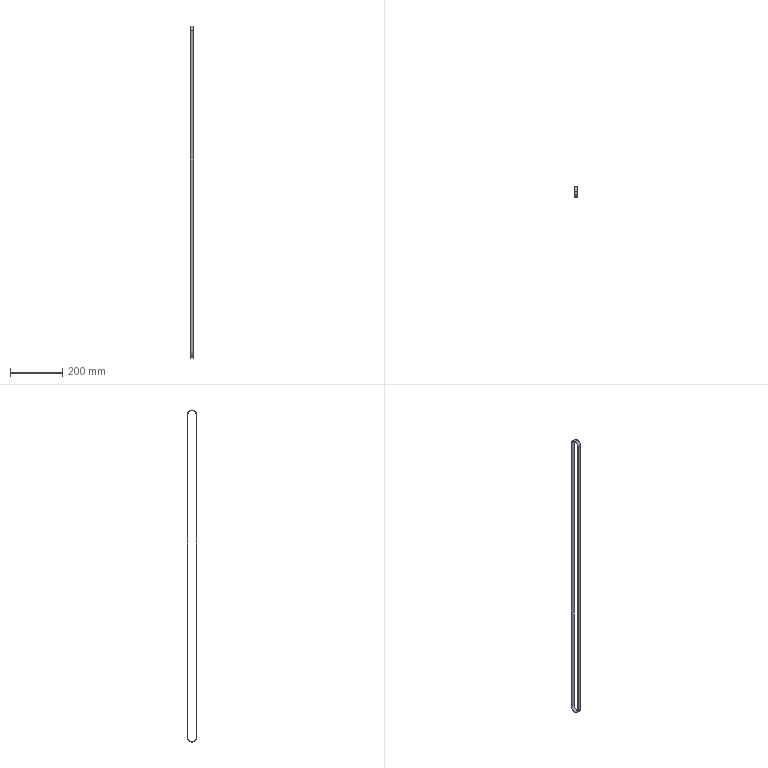Part | STEP file | 0243_101_Belt_050-L-0396A-J | 1 solid | 12 faces | box 13.5 x 37.6 x 1267 mm | volume 69386 mm3 | cylinder 6 | plane 6 | commonest cylinder face diameters 33.6 x3 37.6 x3
STEP:
#1=CARTESIAN_POINT('',(0.,0.,0.));
#2=DIRECTION('',(0.,0.,1.));
#3=DIRECTION('',(1.,0.,0.));
#4=AXIS2_PLACEMENT_3D('',#1,#2,#3);
#5=CARTESIAN_POINT('',(6.75,16.8,0.));
#6=VERTEX_POINT('',#5);
#7=CARTESIAN_POINT('',(-6.75,16.8,0.));
#8=VERTEX_POINT('',#7);
#9=CARTESIAN_POINT('',(6.75,16.8,0.));
#10=DIRECTION('',(-1.,0.,0.));
#11=VECTOR('',#10,1.);
#12=LINE('',#9,#11);
#13=CARTESIAN_POINT('',(6.75,0.,0.));
#14=DIRECTION('',(-1.,0.,0.));
#15=DIRECTION('',(0.,0.,1.));
#16=AXIS2_PLACEMENT_3D('',#13,#14,#15);
#17=CYLINDRICAL_SURFACE('',#16,16.8);
#18=CARTESIAN_POINT('',(1.571,0.));
#19=DIRECTION('',(0.,1.));
#20=VECTOR('',#19,1.);
#21=LINE('',#18,#20);
#22=(GEOMETRIC_REPRESENTATION_CONTEXT(2)PARAMETRIC_REPRESENTATION_CONTEXT()REPRESENTATION_CONTEXT('',''));
#23=DEFINITIONAL_REPRESENTATION('',(#21),#22);
#24=PCURVE('',#17,#23);
#25=CARTESIAN_POINT('',(6.75,16.8,0.));
#26=DIRECTION('',(0.,-1.,0.));
#27=DIRECTION('',(0.,0.,-1.));
#28=AXIS2_PLACEMENT_3D('',#25,#26,#27);
#29=PLANE('',#28);
#30=CARTESIAN_POINT('',(0.,0.));
#31=DIRECTION('',(0.,-1.));
#32=VECTOR('',#31,1.);
#33=LINE('',#30,#32);
#34=(GEOMETRIC_REPRESENTATION_CONTEXT(2)PARAMETRIC_REPRESENTATION_CONTEXT()REPRESENTATION_CONTEXT('',''));
#35=DEFINITIONAL_REPRESENTATION('',(#33),#34);
#36=PCURVE('',#29,#35);
#37=SURFACE_CURVE('',#12,(#24,#36),.PCURVE_S1.);
#38=EDGE_CURVE('',#6,#8,#37,.T.);
#39=ORIENTED_EDGE('',*,*,#38,.T.);
#40=CARTESIAN_POINT('',(-6.75,0.,16.8));
#41=VERTEX_POINT('',#40);
#42=CARTESIAN_POINT('',(-6.75,0.,0.));
#43=DIRECTION('',(1.,0.,0.));
#44=DIRECTION('',(0.,0.,-1.));
#45=AXIS2_PLACEMENT_3D('',#42,#43,#44);
#46=CIRCLE('',#45,16.8);
#47=CARTESIAN_POINT('',(3.142,13.5));
#48=DIRECTION('',(-1.,0.));
#49=VECTOR('',#48,1.);
#50=LINE('',#47,#49);
#51=(GEOMETRIC_REPRESENTATION_CONTEXT(2)PARAMETRIC_REPRESENTATION_CONTEXT()REPRESENTATION_CONTEXT('',''));
#52=DEFINITIONAL_REPRESENTATION('',(#50),#51);
#53=PCURVE('',#17,#52);
#54=CARTESIAN_POINT('',(-6.75,0.,0.));
#55=DIRECTION('',(1.,0.,0.));
#56=DIRECTION('',(0.,0.,-1.));
#57=AXIS2_PLACEMENT_3D('',#54,#55,#56);
#58=PLANE('',#57);
#59=CARTESIAN_POINT('',(0.,0.));
#60=DIRECTION('',(1.,0.));
#61=AXIS2_PLACEMENT_2D('',#59,#60);
#62=CIRCLE('',#61,16.8);
#63=(GEOMETRIC_REPRESENTATION_CONTEXT(2)PARAMETRIC_REPRESENTATION_CONTEXT()REPRESENTATION_CONTEXT('',''));
#64=DEFINITIONAL_REPRESENTATION('',(#62),#63);
#65=PCURVE('',#58,#64);
#66=SURFACE_CURVE('',#46,(#53,#65),.PCURVE_S1.);
#67=EDGE_CURVE('',#8,#41,#66,.T.);
#68=ORIENTED_EDGE('',*,*,#67,.T.);
#69=CARTESIAN_POINT('',(6.75,0.,16.8));
#70=VERTEX_POINT('',#69);
#71=CARTESIAN_POINT('',(6.75,0.,16.8));
#72=DIRECTION('',(-1.,0.,0.));
#73=VECTOR('',#72,1.);
#74=LINE('',#71,#73);
#75=CARTESIAN_POINT('',(0.,0.));
#76=DIRECTION('',(0.,1.));
#77=VECTOR('',#76,1.);
#78=LINE('',#75,#77);
#79=(GEOMETRIC_REPRESENTATION_CONTEXT(2)PARAMETRIC_REPRESENTATION_CONTEXT()REPRESENTATION_CONTEXT('',''));
#80=DEFINITIONAL_REPRESENTATION('',(#78),#79);
#81=PCURVE('',#17,#80);
#82=CARTESIAN_POINT('',(6.75,0.,0.));
#83=DIRECTION('',(-1.,0.,0.));
#84=DIRECTION('',(0.,0.,1.));
#85=AXIS2_PLACEMENT_3D('',#82,#83,#84);
#86=CYLINDRICAL_SURFACE('',#85,16.8);
#87=CARTESIAN_POINT('',(6.283,0.));
#88=DIRECTION('',(0.,1.));
#89=VECTOR('',#88,1.);
#90=LINE('',#87,#89);
#91=(GEOMETRIC_REPRESENTATION_CONTEXT(2)PARAMETRIC_REPRESENTATION_CONTEXT()REPRESENTATION_CONTEXT('',''));
#92=DEFINITIONAL_REPRESENTATION('',(#90),#91);
#93=PCURVE('',#86,#92);
#94=SURFACE_CURVE('',#74,(#81,#93),.PCURVE_S1.);
#95=EDGE_CURVE('',#70,#41,#94,.T.);
#96=ORIENTED_EDGE('',*,*,#95,.F.);
#97=CARTESIAN_POINT('',(6.75,0.,0.));
#98=DIRECTION('',(1.,0.,0.));
#99=DIRECTION('',(0.,0.,-1.));
#100=AXIS2_PLACEMENT_3D('',#97,#98,#99);
#101=CIRCLE('',#100,16.8);
#102=CARTESIAN_POINT('',(3.142,0.));
#103=DIRECTION('',(-1.,0.));
#104=VECTOR('',#103,1.);
#105=LINE('',#102,#104);
#106=(GEOMETRIC_REPRESENTATION_CONTEXT(2)PARAMETRIC_REPRESENTATION_CONTEXT()REPRESENTATION_CONTEXT('',''));
#107=DEFINITIONAL_REPRESENTATION('',(#105),#106);
#108=PCURVE('',#17,#107);
#109=CARTESIAN_POINT('',(6.75,0.,0.));
#110=DIRECTION('',(1.,0.,0.));
#111=DIRECTION('',(0.,0.,-1.));
#112=AXIS2_PLACEMENT_3D('',#109,#110,#111);
#113=PLANE('',#112);
#114=CARTESIAN_POINT('',(0.,0.));
#115=DIRECTION('',(1.,0.));
#116=AXIS2_PLACEMENT_2D('',#114,#115);
#117=CIRCLE('',#116,16.8);
#118=(GEOMETRIC_REPRESENTATION_CONTEXT(2)PARAMETRIC_REPRESENTATION_CONTEXT()REPRESENTATION_CONTEXT('',''));
#119=DEFINITIONAL_REPRESENTATION('',(#117),#118);
#120=PCURVE('',#113,#119);
#121=SURFACE_CURVE('',#101,(#108,#120),.PCURVE_S1.);
#122=EDGE_CURVE('',#6,#70,#121,.T.);
#123=ORIENTED_EDGE('',*,*,#122,.F.);
#124=EDGE_LOOP('',(#39,#68,#96,#123));
#125=FACE_BOUND('',#124,.F.);
#126=ADVANCED_FACE('',(#125),#17,.F.);
#127=CARTESIAN_POINT('',(6.75,0.,18.8));
#128=VERTEX_POINT('',#127);
#129=CARTESIAN_POINT('',(6.75,-18.8,0.));
#130=VERTEX_POINT('',#129);
#131=CARTESIAN_POINT('',(6.75,0.,0.));
#132=DIRECTION('',(1.,0.,0.));
#133=DIRECTION('',(0.,0.,-1.));
#134=AXIS2_PLACEMENT_3D('',#131,#132,#133);
#135=CIRCLE('',#134,18.8);
#136=CARTESIAN_POINT('',(6.75,0.,0.));
#137=DIRECTION('',(-1.,0.,0.));
#138=DIRECTION('',(0.,0.,1.));
#139=AXIS2_PLACEMENT_3D('',#136,#137,#138);
#140=CYLINDRICAL_SURFACE('',#139,18.8);
#141=CARTESIAN_POINT('',(9.425,0.));
#142=DIRECTION('',(-1.,0.));
#143=VECTOR('',#142,1.);
#144=LINE('',#141,#143);
#145=(GEOMETRIC_REPRESENTATION_CONTEXT(2)PARAMETRIC_REPRESENTATION_CONTEXT()REPRESENTATION_CONTEXT('',''));
#146=DEFINITIONAL_REPRESENTATION('',(#144),#145);
#147=PCURVE('',#140,#146);
#148=CARTESIAN_POINT('',(0.,0.));
#149=DIRECTION('',(1.,0.));
#150=AXIS2_PLACEMENT_2D('',#148,#149);
#151=CIRCLE('',#150,18.8);
#152=(GEOMETRIC_REPRESENTATION_CONTEXT(2)PARAMETRIC_REPRESENTATION_CONTEXT()REPRESENTATION_CONTEXT('',''));
#153=DEFINITIONAL_REPRESENTATION('',(#151),#152);
#154=PCURVE('',#113,#153);
#155=SURFACE_CURVE('',#135,(#147,#154),.PCURVE_S1.);
#156=EDGE_CURVE('',#128,#130,#155,.T.);
#157=ORIENTED_EDGE('',*,*,#156,.F.);
#158=CARTESIAN_POINT('',(-6.75,0.,18.8));
#159=VERTEX_POINT('',#158);
#160=CARTESIAN_POINT('',(6.75,0.,18.8));
#161=DIRECTION('',(-1.,0.,0.));
#162=VECTOR('',#161,1.);
#163=LINE('',#160,#162);
#164=CARTESIAN_POINT('',(6.283,0.));
#165=DIRECTION('',(0.,1.));
#166=VECTOR('',#165,1.);
#167=LINE('',#164,#166);
#168=(GEOMETRIC_REPRESENTATION_CONTEXT(2)PARAMETRIC_REPRESENTATION_CONTEXT()REPRESENTATION_CONTEXT('',''));
#169=DEFINITIONAL_REPRESENTATION('',(#167),#168);
#170=PCURVE('',#140,#169);
#171=CARTESIAN_POINT('',(6.75,0.,0.));
#172=DIRECTION('',(-1.,0.,0.));
#173=DIRECTION('',(0.,0.,1.));
#174=AXIS2_PLACEMENT_3D('',#171,#172,#173);
#175=CYLINDRICAL_SURFACE('',#174,18.8);
#176=CARTESIAN_POINT('',(0.,0.));
#177=DIRECTION('',(0.,1.));
#178=VECTOR('',#177,1.);
#179=LINE('',#176,#178);
#180=(GEOMETRIC_REPRESENTATION_CONTEXT(2)PARAMETRIC_REPRESENTATION_CONTEXT()REPRESENTATION_CONTEXT('',''));
#181=DEFINITIONAL_REPRESENTATION('',(#179),#180);
#182=PCURVE('',#175,#181);
#183=SURFACE_CURVE('',#163,(#170,#182),.PCURVE_S1.);
#184=EDGE_CURVE('',#128,#159,#183,.T.);
#185=ORIENTED_EDGE('',*,*,#184,.T.);
#186=CARTESIAN_POINT('',(-6.75,-18.8,0.));
#187=VERTEX_POINT('',#186);
#188=CARTESIAN_POINT('',(-6.75,0.,0.));
#189=DIRECTION('',(1.,0.,0.));
#190=DIRECTION('',(0.,0.,-1.));
#191=AXIS2_PLACEMENT_3D('',#188,#189,#190);
#192=CIRCLE('',#191,18.8);
#193=CARTESIAN_POINT('',(9.425,13.5));
#194=DIRECTION('',(-1.,0.));
#195=VECTOR('',#194,1.);
#196=LINE('',#193,#195);
#197=(GEOMETRIC_REPRESENTATION_CONTEXT(2)PARAMETRIC_REPRESENTATION_CONTEXT()REPRESENTATION_CONTEXT('',''));
#198=DEFINITIONAL_REPRESENTATION('',(#196),#197);
#199=PCURVE('',#140,#198);
#200=CARTESIAN_POINT('',(0.,0.));
#201=DIRECTION('',(1.,0.));
#202=AXIS2_PLACEMENT_2D('',#200,#201);
#203=CIRCLE('',#202,18.8);
#204=(GEOMETRIC_REPRESENTATION_CONTEXT(2)PARAMETRIC_REPRESENTATION_CONTEXT()REPRESENTATION_CONTEXT('',''));
#205=DEFINITIONAL_REPRESENTATION('',(#203),#204);
#206=PCURVE('',#58,#205);
#207=SURFACE_CURVE('',#192,(#199,#206),.PCURVE_S1.);
#208=EDGE_CURVE('',#159,#187,#207,.T.);
#209=ORIENTED_EDGE('',*,*,#208,.T.);
#210=CARTESIAN_POINT('',(6.75,-18.8,0.));
#211=DIRECTION('',(-1.,0.,0.));
#212=VECTOR('',#211,1.);
#213=LINE('',#210,#212);
#214=CARTESIAN_POINT('',(4.712,0.));
#215=DIRECTION('',(0.,1.));
#216=VECTOR('',#215,1.);
#217=LINE('',#214,#216);
#218=(GEOMETRIC_REPRESENTATION_CONTEXT(2)PARAMETRIC_REPRESENTATION_CONTEXT()REPRESENTATION_CONTEXT('',''));
#219=DEFINITIONAL_REPRESENTATION('',(#217),#218);
#220=PCURVE('',#140,#219);
#221=CARTESIAN_POINT('',(6.75,-18.8,-1229.));
#222=DIRECTION('',(0.,1.,0.));
#223=DIRECTION('',(0.,0.,1.));
#224=AXIS2_PLACEMENT_3D('',#221,#222,#223);
#225=PLANE('',#224);
#226=CARTESIAN_POINT('',(1229.,0.));
#227=DIRECTION('',(0.,-1.));
#228=VECTOR('',#227,1.);
#229=LINE('',#226,#228);
#230=(GEOMETRIC_REPRESENTATION_CONTEXT(2)PARAMETRIC_REPRESENTATION_CONTEXT()REPRESENTATION_CONTEXT('',''));
#231=DEFINITIONAL_REPRESENTATION('',(#229),#230);
#232=PCURVE('',#225,#231);
#233=SURFACE_CURVE('',#213,(#220,#232),.PCURVE_S1.);
#234=EDGE_CURVE('',#130,#187,#233,.T.);
#235=ORIENTED_EDGE('',*,*,#234,.F.);
#236=EDGE_LOOP('',(#157,#185,#209,#235));
#237=FACE_BOUND('',#236,.T.);
#238=ADVANCED_FACE('',(#237),#140,.T.);
#239=CARTESIAN_POINT('',(6.75,18.8,0.));
#240=VERTEX_POINT('',#239);
#241=CARTESIAN_POINT('',(6.75,0.,0.));
#242=DIRECTION('',(1.,0.,0.));
#243=DIRECTION('',(0.,0.,-1.));
#244=AXIS2_PLACEMENT_3D('',#241,#242,#243);
#245=CIRCLE('',#244,18.8);
#246=CARTESIAN_POINT('',(0.,0.));
#247=DIRECTION('',(1.,0.));
#248=AXIS2_PLACEMENT_2D('',#246,#247);
#249=CIRCLE('',#248,18.8);
#250=(GEOMETRIC_REPRESENTATION_CONTEXT(2)PARAMETRIC_REPRESENTATION_CONTEXT()REPRESENTATION_CONTEXT('',''));
#251=DEFINITIONAL_REPRESENTATION('',(#249),#250);
#252=PCURVE('',#113,#251);
#253=CARTESIAN_POINT('',(3.142,0.));
#254=DIRECTION('',(-1.,0.));
#255=VECTOR('',#254,1.);
#256=LINE('',#253,#255);
#257=(GEOMETRIC_REPRESENTATION_CONTEXT(2)PARAMETRIC_REPRESENTATION_CONTEXT()REPRESENTATION_CONTEXT('',''));
#258=DEFINITIONAL_REPRESENTATION('',(#256),#257);
#259=PCURVE('',#175,#258);
#260=SURFACE_CURVE('',#245,(#252,#259),.PCURVE_S1.);
#261=EDGE_CURVE('',#240,#128,#260,.T.);
#262=ORIENTED_EDGE('',*,*,#261,.T.);
#263=ORIENTED_EDGE('',*,*,#156,.T.);
#264=CARTESIAN_POINT('',(6.75,-18.8,-1229.));
#265=VERTEX_POINT('',#264);
#266=CARTESIAN_POINT('',(6.75,-18.8,-1229.));
#267=DIRECTION('',(0.,0.,-1.));
#268=VECTOR('',#267,1.);
#269=LINE('',#266,#268);
#270=CARTESIAN_POINT('',(1229.,-18.8));
#271=DIRECTION('',(1.,0.));
#272=VECTOR('',#271,1.);
#273=LINE('',#270,#272);
#274=(GEOMETRIC_REPRESENTATION_CONTEXT(2)PARAMETRIC_REPRESENTATION_CONTEXT()REPRESENTATION_CONTEXT('',''));
#275=DEFINITIONAL_REPRESENTATION('',(#273),#274);
#276=PCURVE('',#113,#275);
#277=CARTESIAN_POINT('',(0.,0.));
#278=DIRECTION('',(-1.,0.));
#279=VECTOR('',#278,1.);
#280=LINE('',#277,#279);
#281=(GEOMETRIC_REPRESENTATION_CONTEXT(2)PARAMETRIC_REPRESENTATION_CONTEXT()REPRESENTATION_CONTEXT('',''));
#282=DEFINITIONAL_REPRESENTATION('',(#280),#281);
#283=PCURVE('',#225,#282);
#284=SURFACE_CURVE('',#269,(#276,#283),.PCURVE_S1.);
#285=EDGE_CURVE('',#130,#265,#284,.T.);
#286=ORIENTED_EDGE('',*,*,#285,.T.);
#287=CARTESIAN_POINT('',(6.75,18.8,-1229.));
#288=VERTEX_POINT('',#287);
#289=CARTESIAN_POINT('',(6.75,0.,-1229.));
#290=DIRECTION('',(1.,0.,0.));
#291=DIRECTION('',(0.,0.,-1.));
#292=AXIS2_PLACEMENT_3D('',#289,#290,#291);
#293=CIRCLE('',#292,18.8);
#294=CARTESIAN_POINT('',(1229.,0.));
#295=DIRECTION('',(1.,0.));
#296=AXIS2_PLACEMENT_2D('',#294,#295);
#297=CIRCLE('',#296,18.8);
#298=(GEOMETRIC_REPRESENTATION_CONTEXT(2)PARAMETRIC_REPRESENTATION_CONTEXT()REPRESENTATION_CONTEXT('',''));
#299=DEFINITIONAL_REPRESENTATION('',(#297),#298);
#300=PCURVE('',#113,#299);
#301=CARTESIAN_POINT('',(6.75,0.,-1229.));
#302=DIRECTION('',(-1.,0.,0.));
#303=DIRECTION('',(0.,0.,1.));
#304=AXIS2_PLACEMENT_3D('',#301,#302,#303);
#305=CYLINDRICAL_SURFACE('',#304,18.8);
#306=CARTESIAN_POINT('',(9.425,0.));
#307=DIRECTION('',(-1.,0.));
#308=VECTOR('',#307,1.);
#309=LINE('',#306,#308);
#310=(GEOMETRIC_REPRESENTATION_CONTEXT(2)PARAMETRIC_REPRESENTATION_CONTEXT()REPRESENTATION_CONTEXT('',''));
#311=DEFINITIONAL_REPRESENTATION('',(#309),#310);
#312=PCURVE('',#305,#311);
#313=SURFACE_CURVE('',#293,(#300,#312),.PCURVE_S1.);
#314=EDGE_CURVE('',#265,#288,#313,.T.);
#315=ORIENTED_EDGE('',*,*,#314,.T.);
#316=CARTESIAN_POINT('',(6.75,18.8,0.));
#317=DIRECTION('',(0.,0.,1.));
#318=VECTOR('',#317,1.);
#319=LINE('',#316,#318);
#320=CARTESIAN_POINT('',(0.,18.8));
#321=DIRECTION('',(-1.,0.));
#322=VECTOR('',#321,1.);
#323=LINE('',#320,#322);
#324=(GEOMETRIC_REPRESENTATION_CONTEXT(2)PARAMETRIC_REPRESENTATION_CONTEXT()REPRESENTATION_CONTEXT('',''));
#325=DEFINITIONAL_REPRESENTATION('',(#323),#324);
#326=PCURVE('',#113,#325);
#327=CARTESIAN_POINT('',(6.75,18.8,0.));
#328=DIRECTION('',(0.,-1.,0.));
#329=DIRECTION('',(0.,0.,-1.));
#330=AXIS2_PLACEMENT_3D('',#327,#328,#329);
#331=PLANE('',#330);
#332=CARTESIAN_POINT('',(0.,0.));
#333=DIRECTION('',(-1.,0.));
#334=VECTOR('',#333,1.);
#335=LINE('',#332,#334);
#336=(GEOMETRIC_REPRESENTATION_CONTEXT(2)PARAMETRIC_REPRESENTATION_CONTEXT()REPRESENTATION_CONTEXT('',''));
#337=DEFINITIONAL_REPRESENTATION('',(#335),#336);
#338=PCURVE('',#331,#337);
#339=SURFACE_CURVE('',#319,(#326,#338),.PCURVE_S1.);
#340=EDGE_CURVE('',#288,#240,#339,.T.);
#341=ORIENTED_EDGE('',*,*,#340,.T.);
#342=EDGE_LOOP('',(#262,#263,#286,#315,#341));
#343=FACE_BOUND('',#342,.T.);
#344=CARTESIAN_POINT('',(6.75,-16.8,0.));
#345=VERTEX_POINT('',#344);
#346=CARTESIAN_POINT('',(6.75,-16.8,-1229.));
#347=VERTEX_POINT('',#346);
#348=CARTESIAN_POINT('',(6.75,-16.8,-1229.));
#349=DIRECTION('',(0.,0.,-1.));
#350=VECTOR('',#349,1.);
#351=LINE('',#348,#350);
#352=CARTESIAN_POINT('',(1229.,-16.8));
#353=DIRECTION('',(1.,0.));
#354=VECTOR('',#353,1.);
#355=LINE('',#352,#354);
#356=(GEOMETRIC_REPRESENTATION_CONTEXT(2)PARAMETRIC_REPRESENTATION_CONTEXT()REPRESENTATION_CONTEXT('',''));
#357=DEFINITIONAL_REPRESENTATION('',(#355),#356);
#358=PCURVE('',#113,#357);
#359=CARTESIAN_POINT('',(6.75,-16.8,-1229.));
#360=DIRECTION('',(0.,1.,0.));
#361=DIRECTION('',(0.,0.,1.));
#362=AXIS2_PLACEMENT_3D('',#359,#360,#361);
#363=PLANE('',#362);
#364=CARTESIAN_POINT('',(0.,0.));
#365=DIRECTION('',(-1.,0.));
#366=VECTOR('',#365,1.);
#367=LINE('',#364,#366);
#368=(GEOMETRIC_REPRESENTATION_CONTEXT(2)PARAMETRIC_REPRESENTATION_CONTEXT()REPRESENTATION_CONTEXT('',''));
#369=DEFINITIONAL_REPRESENTATION('',(#367),#368);
#370=PCURVE('',#363,#369);
#371=SURFACE_CURVE('',#351,(#358,#370),.PCURVE_S1.);
#372=EDGE_CURVE('',#345,#347,#371,.T.);
#373=ORIENTED_EDGE('',*,*,#372,.F.);
#374=CARTESIAN_POINT('',(6.75,0.,0.));
#375=DIRECTION('',(1.,0.,0.));
#376=DIRECTION('',(0.,0.,-1.));
#377=AXIS2_PLACEMENT_3D('',#374,#375,#376);
#378=CIRCLE('',#377,16.8);
#379=CARTESIAN_POINT('',(0.,0.));
#380=DIRECTION('',(1.,0.));
#381=AXIS2_PLACEMENT_2D('',#379,#380);
#382=CIRCLE('',#381,16.8);
#383=(GEOMETRIC_REPRESENTATION_CONTEXT(2)PARAMETRIC_REPRESENTATION_CONTEXT()REPRESENTATION_CONTEXT('',''));
#384=DEFINITIONAL_REPRESENTATION('',(#382),#383);
#385=PCURVE('',#113,#384);
#386=CARTESIAN_POINT('',(9.425,0.));
#387=DIRECTION('',(-1.,0.));
#388=VECTOR('',#387,1.);
#389=LINE('',#386,#388);
#390=(GEOMETRIC_REPRESENTATION_CONTEXT(2)PARAMETRIC_REPRESENTATION_CONTEXT()REPRESENTATION_CONTEXT('',''));
#391=DEFINITIONAL_REPRESENTATION('',(#389),#390);
#392=PCURVE('',#86,#391);
#393=SURFACE_CURVE('',#378,(#385,#392),.PCURVE_S1.);
#394=EDGE_CURVE('',#70,#345,#393,.T.);
#395=ORIENTED_EDGE('',*,*,#394,.F.);
#396=ORIENTED_EDGE('',*,*,#122,.F.);
#397=CARTESIAN_POINT('',(6.75,16.8,-1229.));
#398=VERTEX_POINT('',#397);
#399=CARTESIAN_POINT('',(6.75,16.8,0.));
#400=DIRECTION('',(0.,0.,1.));
#401=VECTOR('',#400,1.);
#402=LINE('',#399,#401);
#403=CARTESIAN_POINT('',(0.,16.8));
#404=DIRECTION('',(-1.,0.));
#405=VECTOR('',#404,1.);
#406=LINE('',#403,#405);
#407=(GEOMETRIC_REPRESENTATION_CONTEXT(2)PARAMETRIC_REPRESENTATION_CONTEXT()REPRESENTATION_CONTEXT('',''));
#408=DEFINITIONAL_REPRESENTATION('',(#406),#407);
#409=PCURVE('',#113,#408);
#410=CARTESIAN_POINT('',(0.,0.));
#411=DIRECTION('',(-1.,0.));
#412=VECTOR('',#411,1.);
#413=LINE('',#410,#412);
#414=(GEOMETRIC_REPRESENTATION_CONTEXT(2)PARAMETRIC_REPRESENTATION_CONTEXT()REPRESENTATION_CONTEXT('',''));
#415=DEFINITIONAL_REPRESENTATION('',(#413),#414);
#416=PCURVE('',#29,#415);
#417=SURFACE_CURVE('',#402,(#409,#416),.PCURVE_S1.);
#418=EDGE_CURVE('',#398,#6,#417,.T.);
#419=ORIENTED_EDGE('',*,*,#418,.F.);
#420=CARTESIAN_POINT('',(6.75,0.,-1229.));
#421=DIRECTION('',(1.,0.,0.));
#422=DIRECTION('',(0.,0.,-1.));
#423=AXIS2_PLACEMENT_3D('',#420,#421,#422);
#424=CIRCLE('',#423,16.8);
#425=CARTESIAN_POINT('',(1229.,0.));
#426=DIRECTION('',(1.,0.));
#427=AXIS2_PLACEMENT_2D('',#425,#426);
#428=CIRCLE('',#427,16.8);
#429=(GEOMETRIC_REPRESENTATION_CONTEXT(2)PARAMETRIC_REPRESENTATION_CONTEXT()REPRESENTATION_CONTEXT('',''));
#430=DEFINITIONAL_REPRESENTATION('',(#428),#429);
#431=PCURVE('',#113,#430);
#432=CARTESIAN_POINT('',(6.75,0.,-1229.));
#433=DIRECTION('',(-1.,0.,0.));
#434=DIRECTION('',(0.,0.,1.));
#435=AXIS2_PLACEMENT_3D('',#432,#433,#434);
#436=CYLINDRICAL_SURFACE('',#435,16.8);
#437=CARTESIAN_POINT('',(9.425,0.));
#438=DIRECTION('',(-1.,0.));
#439=VECTOR('',#438,1.);
#440=LINE('',#437,#439);
#441=(GEOMETRIC_REPRESENTATION_CONTEXT(2)PARAMETRIC_REPRESENTATION_CONTEXT()REPRESENTATION_CONTEXT('',''));
#442=DEFINITIONAL_REPRESENTATION('',(#440),#441);
#443=PCURVE('',#436,#442);
#444=SURFACE_CURVE('',#424,(#431,#443),.PCURVE_S1.);
#445=EDGE_CURVE('',#347,#398,#444,.T.);
#446=ORIENTED_EDGE('',*,*,#445,.F.);
#447=EDGE_LOOP('',(#373,#395,#396,#419,#446));
#448=FACE_BOUND('',#447,.T.);
#449=ADVANCED_FACE('',(#343,#448),#113,.T.);
#450=CARTESIAN_POINT('',(-6.75,18.8,0.));
#451=VERTEX_POINT('',#450);
#452=CARTESIAN_POINT('',(-6.75,0.,0.));
#453=DIRECTION('',(1.,0.,0.));
#454=DIRECTION('',(0.,0.,-1.));
#455=AXIS2_PLACEMENT_3D('',#452,#453,#454);
#456=CIRCLE('',#455,18.8);
#457=CARTESIAN_POINT('',(0.,0.));
#458=DIRECTION('',(1.,0.));
#459=AXIS2_PLACEMENT_2D('',#457,#458);
#460=CIRCLE('',#459,18.8);
#461=(GEOMETRIC_REPRESENTATION_CONTEXT(2)PARAMETRIC_REPRESENTATION_CONTEXT()REPRESENTATION_CONTEXT('',''));
#462=DEFINITIONAL_REPRESENTATION('',(#460),#461);
#463=PCURVE('',#58,#462);
#464=CARTESIAN_POINT('',(3.142,13.5));
#465=DIRECTION('',(-1.,0.));
#466=VECTOR('',#465,1.);
#467=LINE('',#464,#466);
#468=(GEOMETRIC_REPRESENTATION_CONTEXT(2)PARAMETRIC_REPRESENTATION_CONTEXT()REPRESENTATION_CONTEXT('',''));
#469=DEFINITIONAL_REPRESENTATION('',(#467),#468);
#470=PCURVE('',#175,#469);
#471=SURFACE_CURVE('',#456,(#463,#470),.PCURVE_S1.);
#472=EDGE_CURVE('',#451,#159,#471,.T.);
#473=ORIENTED_EDGE('',*,*,#472,.F.);
#474=CARTESIAN_POINT('',(-6.75,18.8,-1229.));
#475=VERTEX_POINT('',#474);
#476=CARTESIAN_POINT('',(-6.75,18.8,0.));
#477=DIRECTION('',(0.,0.,1.));
#478=VECTOR('',#477,1.);
#479=LINE('',#476,#478);
#480=CARTESIAN_POINT('',(0.,18.8));
#481=DIRECTION('',(-1.,0.));
#482=VECTOR('',#481,1.);
#483=LINE('',#480,#482);
#484=(GEOMETRIC_REPRESENTATION_CONTEXT(2)PARAMETRIC_REPRESENTATION_CONTEXT()REPRESENTATION_CONTEXT('',''));
#485=DEFINITIONAL_REPRESENTATION('',(#483),#484);
#486=PCURVE('',#58,#485);
#487=CARTESIAN_POINT('',(0.,-13.5));
#488=DIRECTION('',(-1.,0.));
#489=VECTOR('',#488,1.);
#490=LINE('',#487,#489);
#491=(GEOMETRIC_REPRESENTATION_CONTEXT(2)PARAMETRIC_REPRESENTATION_CONTEXT()REPRESENTATION_CONTEXT('',''));
#492=DEFINITIONAL_REPRESENTATION('',(#490),#491);
#493=PCURVE('',#331,#492);
#494=SURFACE_CURVE('',#479,(#486,#493),.PCURVE_S1.);
#495=EDGE_CURVE('',#475,#451,#494,.T.);
#496=ORIENTED_EDGE('',*,*,#495,.F.);
#497=CARTESIAN_POINT('',(-6.75,-18.8,-1229.));
#498=VERTEX_POINT('',#497);
#499=CARTESIAN_POINT('',(-6.75,0.,-1229.));
#500=DIRECTION('',(1.,0.,0.));
#501=DIRECTION('',(0.,0.,-1.));
#502=AXIS2_PLACEMENT_3D('',#499,#500,#501);
#503=CIRCLE('',#502,18.8);
#504=CARTESIAN_POINT('',(1229.,0.));
#505=DIRECTION('',(1.,0.));
#506=AXIS2_PLACEMENT_2D('',#504,#505);
#507=CIRCLE('',#506,18.8);
#508=(GEOMETRIC_REPRESENTATION_CONTEXT(2)PARAMETRIC_REPRESENTATION_CONTEXT()REPRESENTATION_CONTEXT('',''));
#509=DEFINITIONAL_REPRESENTATION('',(#507),#508);
#510=PCURVE('',#58,#509);
#511=CARTESIAN_POINT('',(9.425,13.5));
#512=DIRECTION('',(-1.,0.));
#513=VECTOR('',#512,1.);
#514=LINE('',#511,#513);
#515=(GEOMETRIC_REPRESENTATION_CONTEXT(2)PARAMETRIC_REPRESENTATION_CONTEXT()REPRESENTATION_CONTEXT('',''));
#516=DEFINITIONAL_REPRESENTATION('',(#514),#515);
#517=PCURVE('',#305,#516);
#518=SURFACE_CURVE('',#503,(#510,#517),.PCURVE_S1.);
#519=EDGE_CURVE('',#498,#475,#518,.T.);
#520=ORIENTED_EDGE('',*,*,#519,.F.);
#521=CARTESIAN_POINT('',(-6.75,-18.8,-1229.));
#522=DIRECTION('',(0.,0.,-1.));
#523=VECTOR('',#522,1.);
#524=LINE('',#521,#523);
#525=CARTESIAN_POINT('',(1229.,-18.8));
#526=DIRECTION('',(1.,0.));
#527=VECTOR('',#526,1.);
#528=LINE('',#525,#527);
#529=(GEOMETRIC_REPRESENTATION_CONTEXT(2)PARAMETRIC_REPRESENTATION_CONTEXT()REPRESENTATION_CONTEXT('',''));
#530=DEFINITIONAL_REPRESENTATION('',(#528),#529);
#531=PCURVE('',#58,#530);
#532=CARTESIAN_POINT('',(0.,-13.5));
#533=DIRECTION('',(-1.,0.));
#534=VECTOR('',#533,1.);
#535=LINE('',#532,#534);
#536=(GEOMETRIC_REPRESENTATION_CONTEXT(2)PARAMETRIC_REPRESENTATION_CONTEXT()REPRESENTATION_CONTEXT('',''));
#537=DEFINITIONAL_REPRESENTATION('',(#535),#536);
#538=PCURVE('',#225,#537);
#539=SURFACE_CURVE('',#524,(#531,#538),.PCURVE_S1.);
#540=EDGE_CURVE('',#187,#498,#539,.T.);
#541=ORIENTED_EDGE('',*,*,#540,.F.);
#542=ORIENTED_EDGE('',*,*,#208,.F.);
#543=EDGE_LOOP('',(#473,#496,#520,#541,#542));
#544=FACE_BOUND('',#543,.T.);
#545=ORIENTED_EDGE('',*,*,#67,.T.);
#546=CARTESIAN_POINT('',(-6.75,-16.8,0.));
#547=VERTEX_POINT('',#546);
#548=CARTESIAN_POINT('',(-6.75,0.,0.));
#549=DIRECTION('',(1.,0.,0.));
#550=DIRECTION('',(0.,0.,-1.));
#551=AXIS2_PLACEMENT_3D('',#548,#549,#550);
#552=CIRCLE('',#551,16.8);
#553=CARTESIAN_POINT('',(0.,0.));
#554=DIRECTION('',(1.,0.));
#555=AXIS2_PLACEMENT_2D('',#553,#554);
#556=CIRCLE('',#555,16.8);
#557=(GEOMETRIC_REPRESENTATION_CONTEXT(2)PARAMETRIC_REPRESENTATION_CONTEXT()REPRESENTATION_CONTEXT('',''));
#558=DEFINITIONAL_REPRESENTATION('',(#556),#557);
#559=PCURVE('',#58,#558);
#560=CARTESIAN_POINT('',(9.425,13.5));
#561=DIRECTION('',(-1.,0.));
#562=VECTOR('',#561,1.);
#563=LINE('',#560,#562);
#564=(GEOMETRIC_REPRESENTATION_CONTEXT(2)PARAMETRIC_REPRESENTATION_CONTEXT()REPRESENTATION_CONTEXT('',''));
#565=DEFINITIONAL_REPRESENTATION('',(#563),#564);
#566=PCURVE('',#86,#565);
#567=SURFACE_CURVE('',#552,(#559,#566),.PCURVE_S1.);
#568=EDGE_CURVE('',#41,#547,#567,.T.);
#569=ORIENTED_EDGE('',*,*,#568,.T.);
#570=CARTESIAN_POINT('',(-6.75,-16.8,-1229.));
#571=VERTEX_POINT('',#570);
#572=CARTESIAN_POINT('',(-6.75,-16.8,-1229.));
#573=DIRECTION('',(0.,0.,-1.));
#574=VECTOR('',#573,1.);
#575=LINE('',#572,#574);
#576=CARTESIAN_POINT('',(1229.,-16.8));
#577=DIRECTION('',(1.,0.));
#578=VECTOR('',#577,1.);
#579=LINE('',#576,#578);
#580=(GEOMETRIC_REPRESENTATION_CONTEXT(2)PARAMETRIC_REPRESENTATION_CONTEXT()REPRESENTATION_CONTEXT('',''));
#581=DEFINITIONAL_REPRESENTATION('',(#579),#580);
#582=PCURVE('',#58,#581);
#583=CARTESIAN_POINT('',(0.,-13.5));
#584=DIRECTION('',(-1.,0.));
#585=VECTOR('',#584,1.);
#586=LINE('',#583,#585);
#587=(GEOMETRIC_REPRESENTATION_CONTEXT(2)PARAMETRIC_REPRESENTATION_CONTEXT()REPRESENTATION_CONTEXT('',''));
#588=DEFINITIONAL_REPRESENTATION('',(#586),#587);
#589=PCURVE('',#363,#588);
#590=SURFACE_CURVE('',#575,(#582,#589),.PCURVE_S1.);
#591=EDGE_CURVE('',#547,#571,#590,.T.);
#592=ORIENTED_EDGE('',*,*,#591,.T.);
#593=CARTESIAN_POINT('',(-6.75,16.8,-1229.));
#594=VERTEX_POINT('',#593);
#595=CARTESIAN_POINT('',(-6.75,0.,-1229.));
#596=DIRECTION('',(1.,0.,0.));
#597=DIRECTION('',(0.,0.,-1.));
#598=AXIS2_PLACEMENT_3D('',#595,#596,#597);
#599=CIRCLE('',#598,16.8);
#600=CARTESIAN_POINT('',(1229.,0.));
#601=DIRECTION('',(1.,0.));
#602=AXIS2_PLACEMENT_2D('',#600,#601);
#603=CIRCLE('',#602,16.8);
#604=(GEOMETRIC_REPRESENTATION_CONTEXT(2)PARAMETRIC_REPRESENTATION_CONTEXT()REPRESENTATION_CONTEXT('',''));
#605=DEFINITIONAL_REPRESENTATION('',(#603),#604);
#606=PCURVE('',#58,#605);
#607=CARTESIAN_POINT('',(9.425,13.5));
#608=DIRECTION('',(-1.,0.));
#609=VECTOR('',#608,1.);
#610=LINE('',#607,#609);
#611=(GEOMETRIC_REPRESENTATION_CONTEXT(2)PARAMETRIC_REPRESENTATION_CONTEXT()REPRESENTATION_CONTEXT('',''));
#612=DEFINITIONAL_REPRESENTATION('',(#610),#611);
#613=PCURVE('',#436,#612);
#614=SURFACE_CURVE('',#599,(#606,#613),.PCURVE_S1.);
#615=EDGE_CURVE('',#571,#594,#614,.T.);
#616=ORIENTED_EDGE('',*,*,#615,.T.);
#617=CARTESIAN_POINT('',(-6.75,16.8,0.));
#618=DIRECTION('',(0.,0.,1.));
#619=VECTOR('',#618,1.);
#620=LINE('',#617,#619);
#621=CARTESIAN_POINT('',(0.,16.8));
#622=DIRECTION('',(-1.,0.));
#623=VECTOR('',#622,1.);
#624=LINE('',#621,#623);
#625=(GEOMETRIC_REPRESENTATION_CONTEXT(2)PARAMETRIC_REPRESENTATION_CONTEXT()REPRESENTATION_CONTEXT('',''));
#626=DEFINITIONAL_REPRESENTATION('',(#624),#625);
#627=PCURVE('',#58,#626);
#628=CARTESIAN_POINT('',(0.,-13.5));
#629=DIRECTION('',(-1.,0.));
#630=VECTOR('',#629,1.);
#631=LINE('',#628,#630);
#632=(GEOMETRIC_REPRESENTATION_CONTEXT(2)PARAMETRIC_REPRESENTATION_CONTEXT()REPRESENTATION_CONTEXT('',''));
#633=DEFINITIONAL_REPRESENTATION('',(#631),#632);
#634=PCURVE('',#29,#633);
#635=SURFACE_CURVE('',#620,(#627,#634),.PCURVE_S1.);
#636=EDGE_CURVE('',#594,#8,#635,.T.);
#637=ORIENTED_EDGE('',*,*,#636,.T.);
#638=EDGE_LOOP('',(#545,#569,#592,#616,#637));
#639=FACE_BOUND('',#638,.T.);
#640=ADVANCED_FACE('',(#544,#639),#58,.F.);
#641=ORIENTED_EDGE('',*,*,#184,.F.);
#642=ORIENTED_EDGE('',*,*,#261,.F.);
#643=CARTESIAN_POINT('',(6.75,18.8,0.));
#644=DIRECTION('',(-1.,0.,0.));
#645=VECTOR('',#644,1.);
#646=LINE('',#643,#645);
#647=CARTESIAN_POINT('',(1.571,0.));
#648=DIRECTION('',(0.,1.));
#649=VECTOR('',#648,1.);
#650=LINE('',#647,#649);
#651=(GEOMETRIC_REPRESENTATION_CONTEXT(2)PARAMETRIC_REPRESENTATION_CONTEXT()REPRESENTATION_CONTEXT('',''));
#652=DEFINITIONAL_REPRESENTATION('',(#650),#651);
#653=PCURVE('',#175,#652);
#654=CARTESIAN_POINT('',(0.,0.));
#655=DIRECTION('',(0.,-1.));
#656=VECTOR('',#655,1.);
#657=LINE('',#654,#656);
#658=(GEOMETRIC_REPRESENTATION_CONTEXT(2)PARAMETRIC_REPRESENTATION_CONTEXT()REPRESENTATION_CONTEXT('',''));
#659=DEFINITIONAL_REPRESENTATION('',(#657),#658);
#660=PCURVE('',#331,#659);
#661=SURFACE_CURVE('',#646,(#653,#660),.PCURVE_S1.);
#662=EDGE_CURVE('',#240,#451,#661,.T.);
#663=ORIENTED_EDGE('',*,*,#662,.T.);
#664=ORIENTED_EDGE('',*,*,#472,.T.);
#665=EDGE_LOOP('',(#641,#642,#663,#664));
#666=FACE_BOUND('',#665,.T.);
#667=ADVANCED_FACE('',(#666),#175,.T.);
#668=ORIENTED_EDGE('',*,*,#540,.T.);
#669=CARTESIAN_POINT('',(6.75,-18.8,-1229.));
#670=DIRECTION('',(-1.,0.,0.));
#671=VECTOR('',#670,1.);
#672=LINE('',#669,#671);
#673=CARTESIAN_POINT('',(0.,0.));
#674=DIRECTION('',(0.,-1.));
#675=VECTOR('',#674,1.);
#676=LINE('',#673,#675);
#677=(GEOMETRIC_REPRESENTATION_CONTEXT(2)PARAMETRIC_REPRESENTATION_CONTEXT()REPRESENTATION_CONTEXT('',''));
#678=DEFINITIONAL_REPRESENTATION('',(#676),#677);
#679=PCURVE('',#225,#678);
#680=CARTESIAN_POINT('',(4.712,0.));
#681=DIRECTION('',(0.,1.));
#682=VECTOR('',#681,1.);
#683=LINE('',#680,#682);
#684=(GEOMETRIC_REPRESENTATION_CONTEXT(2)PARAMETRIC_REPRESENTATION_CONTEXT()REPRESENTATION_CONTEXT('',''));
#685=DEFINITIONAL_REPRESENTATION('',(#683),#684);
#686=PCURVE('',#305,#685);
#687=SURFACE_CURVE('',#672,(#679,#686),.PCURVE_S1.);
#688=EDGE_CURVE('',#265,#498,#687,.T.);
#689=ORIENTED_EDGE('',*,*,#688,.F.);
#690=ORIENTED_EDGE('',*,*,#285,.F.);
#691=ORIENTED_EDGE('',*,*,#234,.T.);
#692=EDGE_LOOP('',(#668,#689,#690,#691));
#693=FACE_BOUND('',#692,.T.);
#694=ADVANCED_FACE('',(#693),#225,.F.);
#695=ORIENTED_EDGE('',*,*,#519,.T.);
#696=CARTESIAN_POINT('',(6.75,18.8,-1229.));
#697=DIRECTION('',(-1.,0.,0.));
#698=VECTOR('',#697,1.);
#699=LINE('',#696,#698);
#700=CARTESIAN_POINT('',(1.571,0.));
#701=DIRECTION('',(0.,1.));
#702=VECTOR('',#701,1.);
#703=LINE('',#700,#702);
#704=(GEOMETRIC_REPRESENTATION_CONTEXT(2)PARAMETRIC_REPRESENTATION_CONTEXT()REPRESENTATION_CONTEXT('',''));
#705=DEFINITIONAL_REPRESENTATION('',(#703),#704);
#706=PCURVE('',#305,#705);
#707=CARTESIAN_POINT('',(1229.,0.));
#708=DIRECTION('',(0.,-1.));
#709=VECTOR('',#708,1.);
#710=LINE('',#707,#709);
#711=(GEOMETRIC_REPRESENTATION_CONTEXT(2)PARAMETRIC_REPRESENTATION_CONTEXT()REPRESENTATION_CONTEXT('',''));
#712=DEFINITIONAL_REPRESENTATION('',(#710),#711);
#713=PCURVE('',#331,#712);
#714=SURFACE_CURVE('',#699,(#706,#713),.PCURVE_S1.);
#715=EDGE_CURVE('',#288,#475,#714,.T.);
#716=ORIENTED_EDGE('',*,*,#715,.F.);
#717=ORIENTED_EDGE('',*,*,#314,.F.);
#718=ORIENTED_EDGE('',*,*,#688,.T.);
#719=EDGE_LOOP('',(#695,#716,#717,#718));
#720=FACE_BOUND('',#719,.T.);
#721=ADVANCED_FACE('',(#720),#305,.T.);
#722=ORIENTED_EDGE('',*,*,#495,.T.);
#723=ORIENTED_EDGE('',*,*,#662,.F.);
#724=ORIENTED_EDGE('',*,*,#340,.F.);
#725=ORIENTED_EDGE('',*,*,#715,.T.);
#726=EDGE_LOOP('',(#722,#723,#724,#725));
#727=FACE_BOUND('',#726,.T.);
#728=ADVANCED_FACE('',(#727),#331,.F.);
#729=ORIENTED_EDGE('',*,*,#568,.T.);
#730=CARTESIAN_POINT('',(6.75,-16.8,0.));
#731=DIRECTION('',(-1.,0.,0.));
#732=VECTOR('',#731,1.);
#733=LINE('',#730,#732);
#734=CARTESIAN_POINT('',(4.712,0.));
#735=DIRECTION('',(0.,1.));
#736=VECTOR('',#735,1.);
#737=LINE('',#734,#736);
#738=(GEOMETRIC_REPRESENTATION_CONTEXT(2)PARAMETRIC_REPRESENTATION_CONTEXT()REPRESENTATION_CONTEXT('',''));
#739=DEFINITIONAL_REPRESENTATION('',(#737),#738);
#740=PCURVE('',#86,#739);
#741=CARTESIAN_POINT('',(1229.,0.));
#742=DIRECTION('',(0.,-1.));
#743=VECTOR('',#742,1.);
#744=LINE('',#741,#743);
#745=(GEOMETRIC_REPRESENTATION_CONTEXT(2)PARAMETRIC_REPRESENTATION_CONTEXT()REPRESENTATION_CONTEXT('',''));
#746=DEFINITIONAL_REPRESENTATION('',(#744),#745);
#747=PCURVE('',#363,#746);
#748=SURFACE_CURVE('',#733,(#740,#747),.PCURVE_S1.);
#749=EDGE_CURVE('',#345,#547,#748,.T.);
#750=ORIENTED_EDGE('',*,*,#749,.F.);
#751=ORIENTED_EDGE('',*,*,#394,.F.);
#752=ORIENTED_EDGE('',*,*,#95,.T.);
#753=EDGE_LOOP('',(#729,#750,#751,#752));
#754=FACE_BOUND('',#753,.F.);
#755=ADVANCED_FACE('',(#754),#86,.F.);
#756=ORIENTED_EDGE('',*,*,#591,.F.);
#757=ORIENTED_EDGE('',*,*,#749,.F.);
#758=ORIENTED_EDGE('',*,*,#372,.T.);
#759=CARTESIAN_POINT('',(6.75,-16.8,-1229.));
#760=DIRECTION('',(-1.,0.,0.));
#761=VECTOR('',#760,1.);
#762=LINE('',#759,#761);
#763=CARTESIAN_POINT('',(0.,0.));
#764=DIRECTION('',(0.,-1.));
#765=VECTOR('',#764,1.);
#766=LINE('',#763,#765);
#767=(GEOMETRIC_REPRESENTATION_CONTEXT(2)PARAMETRIC_REPRESENTATION_CONTEXT()REPRESENTATION_CONTEXT('',''));
#768=DEFINITIONAL_REPRESENTATION('',(#766),#767);
#769=PCURVE('',#363,#768);
#770=CARTESIAN_POINT('',(4.712,0.));
#771=DIRECTION('',(0.,1.));
#772=VECTOR('',#771,1.);
#773=LINE('',#770,#772);
#774=(GEOMETRIC_REPRESENTATION_CONTEXT(2)PARAMETRIC_REPRESENTATION_CONTEXT()REPRESENTATION_CONTEXT('',''));
#775=DEFINITIONAL_REPRESENTATION('',(#773),#774);
#776=PCURVE('',#436,#775);
#777=SURFACE_CURVE('',#762,(#769,#776),.PCURVE_S1.);
#778=EDGE_CURVE('',#347,#571,#777,.T.);
#779=ORIENTED_EDGE('',*,*,#778,.T.);
#780=EDGE_LOOP('',(#756,#757,#758,#779));
#781=FACE_BOUND('',#780,.T.);
#782=ADVANCED_FACE('',(#781),#363,.T.);
#783=CARTESIAN_POINT('',(6.75,16.8,-1229.));
#784=DIRECTION('',(-1.,0.,0.));
#785=VECTOR('',#784,1.);
#786=LINE('',#783,#785);
#787=CARTESIAN_POINT('',(1.571,0.));
#788=DIRECTION('',(0.,1.));
#789=VECTOR('',#788,1.);
#790=LINE('',#787,#789);
#791=(GEOMETRIC_REPRESENTATION_CONTEXT(2)PARAMETRIC_REPRESENTATION_CONTEXT()REPRESENTATION_CONTEXT('',''));
#792=DEFINITIONAL_REPRESENTATION('',(#790),#791);
#793=PCURVE('',#436,#792);
#794=CARTESIAN_POINT('',(1229.,0.));
#795=DIRECTION('',(0.,-1.));
#796=VECTOR('',#795,1.);
#797=LINE('',#794,#796);
#798=(GEOMETRIC_REPRESENTATION_CONTEXT(2)PARAMETRIC_REPRESENTATION_CONTEXT()REPRESENTATION_CONTEXT('',''));
#799=DEFINITIONAL_REPRESENTATION('',(#797),#798);
#800=PCURVE('',#29,#799);
#801=SURFACE_CURVE('',#786,(#793,#800),.PCURVE_S1.);
#802=EDGE_CURVE('',#398,#594,#801,.T.);
#803=ORIENTED_EDGE('',*,*,#802,.F.);
#804=ORIENTED_EDGE('',*,*,#445,.F.);
#805=ORIENTED_EDGE('',*,*,#778,.T.);
#806=ORIENTED_EDGE('',*,*,#615,.T.);
#807=EDGE_LOOP('',(#803,#804,#805,#806));
#808=FACE_BOUND('',#807,.F.);
#809=ADVANCED_FACE('',(#808),#436,.F.);
#810=ORIENTED_EDGE('',*,*,#636,.F.);
#811=ORIENTED_EDGE('',*,*,#802,.F.);
#812=ORIENTED_EDGE('',*,*,#418,.T.);
#813=ORIENTED_EDGE('',*,*,#38,.T.);
#814=EDGE_LOOP('',(#810,#811,#812,#813));
#815=FACE_BOUND('',#814,.T.);
#816=ADVANCED_FACE('',(#815),#29,.T.);
#817=CLOSED_SHELL('',(#126,#238,#449,#640,#667,#694,#721,#728,#755,#782,#809,#816));
#818=MANIFOLD_SOLID_BREP('',#817);
#819=(LENGTH_UNIT()NAMED_UNIT(*)SI_UNIT(.MILLI.,.METRE.));
#820=UNCERTAINTY_MEASURE_WITH_UNIT(LENGTH_MEASURE(0.0000001),#819,'','');
#821=(NAMED_UNIT(*)PLANE_ANGLE_UNIT()SI_UNIT($,.RADIAN.));
#822=(NAMED_UNIT(*)SI_UNIT($,.STERADIAN.)SOLID_ANGLE_UNIT());
#823=(GEOMETRIC_REPRESENTATION_CONTEXT(3)GLOBAL_UNCERTAINTY_ASSIGNED_CONTEXT((#820))GLOBAL_UNIT_ASSIGNED_CONTEXT((#819,#821,#822))REPRESENTATION_CONTEXT('',''));
#824=ADVANCED_BREP_SHAPE_REPRESENTATION('',(#4,#818),#823);